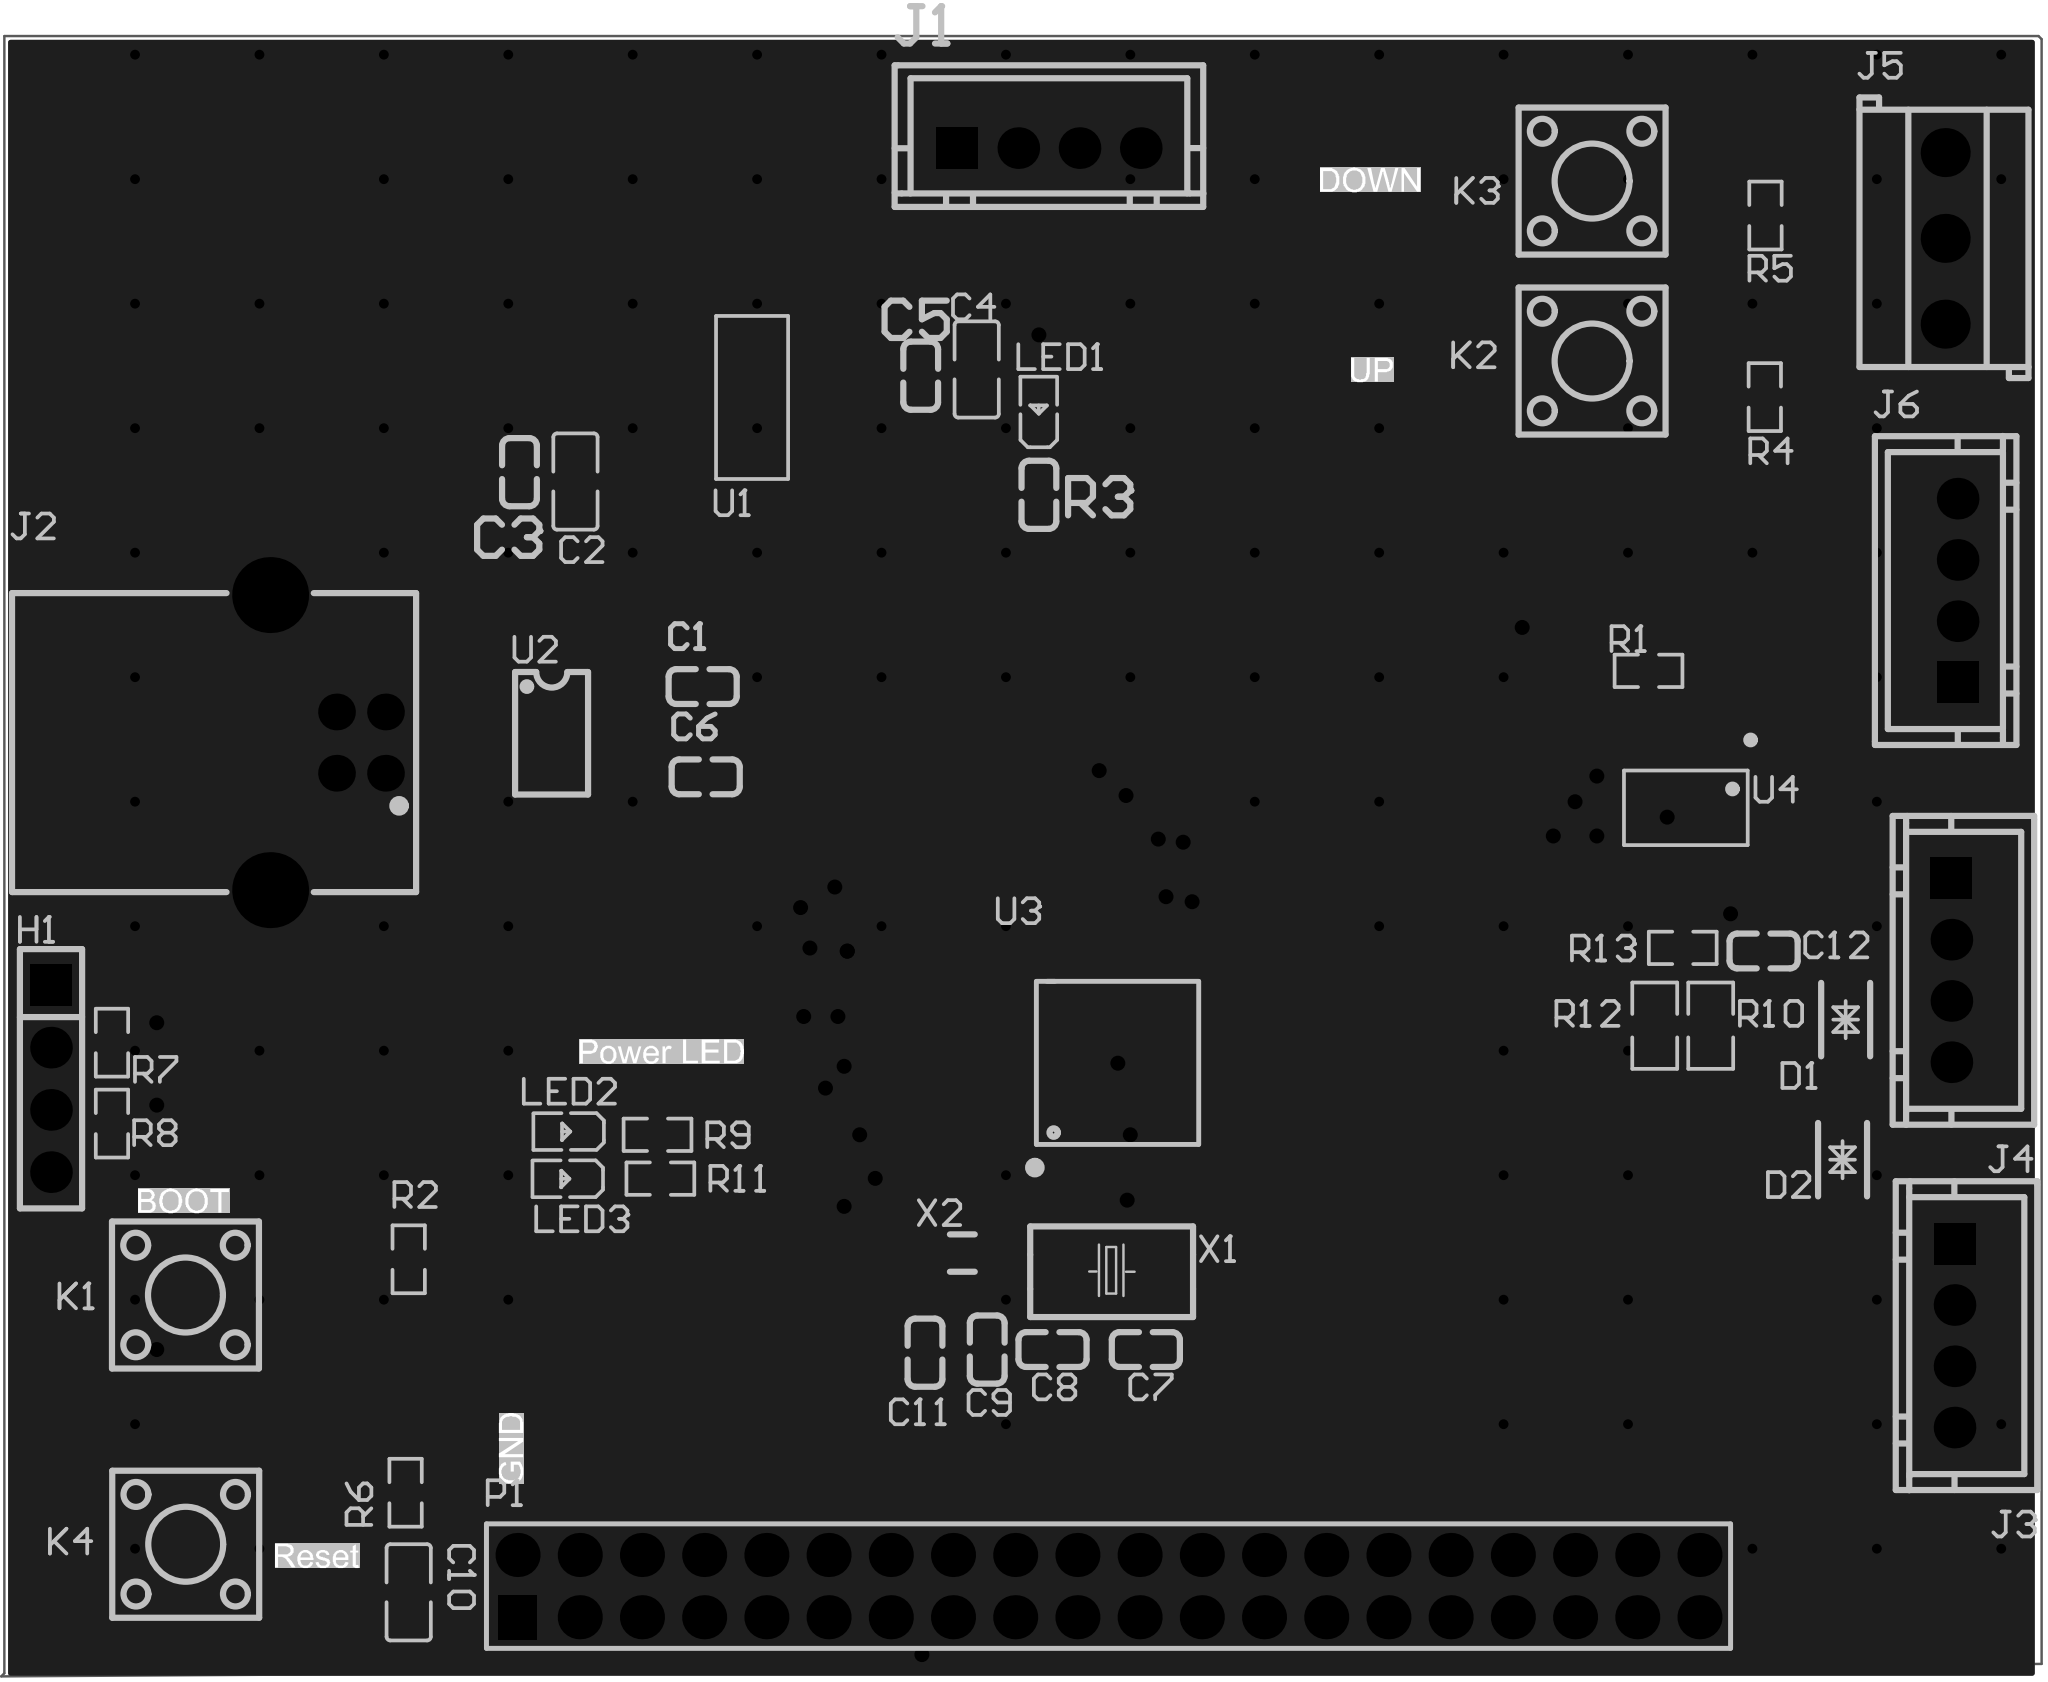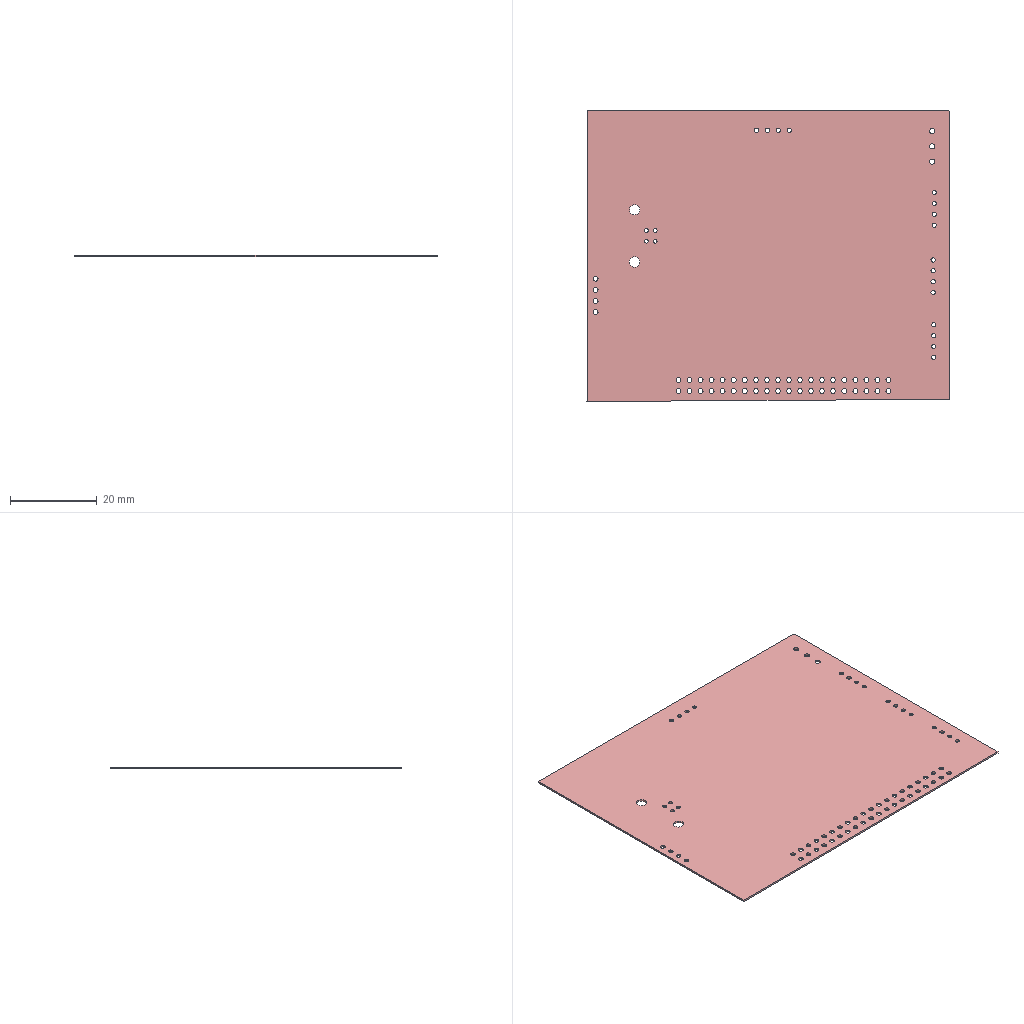Circuit board layout | Altium Designer | box 83.3 x 66.9 x 0.4 mm
Layer stack:
# Altium Designer layer stack of  (unit mm; dielectric type: 0 none, 1 core, 2 prepreg, 3 surface material)
index,name,kind,layer,copper_thickness_mm,dielectric_type,dielectric_thickness_mm,dielectric_material,dielectric_constant
0,Top Paste Mask Layer,other,,,,,,
1,Top Silkscreen Layer,other,,,,,,
2,Top Solder Mask Layer,dielectric,,,3,0.0102,Solder Resist,3.5
3,Top Layer,copper,Top Layer,0.0356,,,,
4,Dielectric 1,dielectric,,,3,0.32,FR-4,4.8
5,Bottom Layer,copper,Bottom Layer,0.0356,,,,
6,Bottom Solder Mask Layer,dielectric,,,3,0.0102,Solder Resist,3.5
7,Bottom Silkscreen Layer,other,,,,,,
8,Bottom Paste Mask Layer,other,,,,,,
# drill layer pairs: low layer,high layer
drill_pair,Top Layer,Bottom Layer
Part placement:
Designator,Comment,Layer,Footprint,Center-X(mm),Center-Y(mm),Rotation
C5,CC0603KRX7R9BB104,TopLayer,C0603_-_duplicate,113.743,129.398,270
C3,CC0603KRX7R9BB104,TopLayer,C0603_-_duplicate,97.36,125.461,270
R3,0603WAF1001T5E,TopLayer,C0603_-_duplicate,118.57,124.538,90
J1,XH-4A,TopLayer,XH-4A,118.979,138.684,0
C6,CC0603KRX7R9BB104,TopLayer,C0603_-_duplicate,104.964,113.03,180
C1,CC0603KRX7R9BB104,TopLayer,C0603_-_duplicate,104.84,116.713,0
X2,X50328MSB2GI,TopLayer,FC-135R_L3.2-W1.5,115.443,93.599,180
X1,Q13FC1350000400,TopLayer,CRYSTAL-SMD_L5.0-W3.2,121.539,92.837,180
U1,AMS1117-3.3,TopLayer,SOT-223-3_L6.5-W3.4-P2.30-LS7.0-BR,106.758,128.509,180
U4,SP3485EEN,TopLayer,485SOP-8_L5.0-W4.0-P1.27-LS6.0-BL,144.985,111.767,180
U3,STM32F103C8T6,TopLayer,LQFP-48_L7.0-W7.0-P0.50-LS9.0-BL,121.793,101.346,0
U2,CH340N_C2977777,TopLayer,SOP-8_L4.9-W3.9-P1.27-LS6.0-BL,98.679,114.808,270
R11,0603WAF1001T5E,TopLayer,R06031k,103.113,96.636,180
R8,0603WAF4701T5E,TopLayer,R06034.7k,80.721,98.882,90
R7,0603WAF4701T5E,TopLayer,R06034.7k,80.721,102.184,90
R9,0603WAF1001T5E,TopLayer,R06031k,102.997,98.425,180
R5,0603WAF1002T5E,TopLayer,电阻R0603,148.237,135.933,270
R2,0603WAF1002T5E,TopLayer,电阻R0603,92.837,93.345,270
R6,0603WAF1002T5E,TopLayer,电阻R0603,92.71,83.82,270
R4,0603WAF1002T5E,TopLayer,电阻R0603,148.209,128.524,270
R1,0603WAF1002T5E,TopLayer,电阻R0603,143.461,117.355,180
R12,0805W8F200JT5E,TopLayer,R0805,143.715,102.877,270
R13,0603WAF1200T5E,TopLayer,R0603_-_duplicate,144.858,106.052,0
R10,0805W8F200JT5E,TopLayer,R0805,146.001,102.877,270
P1,Header-Male-2.54_2x20,TopLayer,HDR-TH_40P-P2.54-V-M-R2-C20-S2.54,121.412,80.01,0
LED3,FC-D1608HGK-572C,TopLayer,LED0603-RD,99.282,96.636,180
LED2,FC-D1608HGK-572C,TopLayer,LED0603-RD,99.318,98.563,180
LED1,FC-D1608HGK-572C,TopLayer,LED0603-RD,118.57,127.967,90
K3,KH-6X6X5H-STM,TopLayer,复位按键,141.157,137.339,180
K4,KH-6X6X5H-STM,TopLayer,复位按键,83.733,81.719,180
K1,KH-6X6X5H-STM,TopLayer,按键,83.722,91.888,0
K2,KH-6X6X5H-STM,TopLayer,复位按键,141.157,129.996,180
J5,KF350-3.5-3P,TopLayer,KF350-3.5-3P,155.575,135.001,90
J6,XH-4A,TopLayer,XH-4A,156.083,120.63,90
J4,XH-4A,TopLayer,XH-4A,155.829,105.136,270
J3,XH-4A,TopLayer,XH-4A,155.956,90.23,270
J2,USB-B-Female-90,TopLayer,USB-B_TH_USB-B-FEMALE-90,89.535,114.427,270
H1,PM254V-11-04-H85,TopLayer,排母4p,78.232,100.711,270
D2,SMF6.0CA_C2990473,TopLayer,瞬态二极管,151.384,97.409,90
D1,SMF6.0CA_C2990473,TopLayer,瞬态二极管,151.511,103.124,90
C11,CL10C200JB8NNNC,TopLayer,C0603c20pf,113.919,89.535,90
C9,CL10C200JB8NNNC,TopLayer,C0603c20pf,116.459,89.662,90
C8,CL10C200JB8NNNC,TopLayer,C0603c20pf,119.126,89.662,0
C10,CL21A106KAYNNNE,TopLayer,C0805,92.837,79.756,90
C7,CL10C200JB8NNNC,TopLayer,C0603c20pf,122.936,89.662,0
C2,CL21A106KAYNNNE,TopLayer,C0805,99.646,125.08,90
C4,CL21A106KAYNNNE,TopLayer,C0805,116.029,129.652,270
C12,CC0603KRX7R9BB104,TopLayer,C0603_-_duplicate,148.16,105.925,0
Pad and via stacks:
# Altium Designer via and pad stacks of  (unit mm). Each distinct definition once, with the count of objects using it.
# via: kind,start_layer,end_layer,hole_mm,diameter_mm,mode(0 simple;1 top-mid-bottom;2 full stack),diameter_per_layer,count,example_net
# pad: kind,layer,hole_mm,hole_type(0 round;1 square;2 slot),plating,top_size,top_shape(1 round;2 rect;3 octagon;9 rounded rect),mid_size,bottom_size,mode,footprint,size_per_layer,count,example
pad,Top Layer,0,0,plated,0.8x0.9,2,0.8x0.9,0.8x0.9,0,C0603 - duplicate,,12,C5.2
pad,Top Layer,0,0,plated,1.8x1,2,1.8x1,1.8x1,0,FC-135R_L3.2-W1.5,,2,X2.2
pad,Top Layer,0,0,plated,1.9x2.4,2,1.9x2.4,1.9x2.4,0,CRYSTAL-SMD_L5.0-W3.2,,2,X1.1
pad,Top Layer,0,0,plated,2.34x3.6,2,2.34x3.6,2.34x3.6,0,SOT-223-3_L6.5-W3.4-P2.30-LS7.0-BR,,1,U1.4
pad,Top Layer,0,0,plated,2.5x1.1,2,2.5x1.1,2.5x1.1,0,SOT-223-3_L6.5-W3.4-P2.30-LS7.0-BR,,3,U1.3
pad,Top Layer,0,0,plated,0.574x2.035,1,0.574x2.035,0.574x2.035,0,485SOP-8_L5.0-W4.0-P1.27-LS6.0-BL,,8,U4.1
pad,Top Layer,0,0,plated,0.27x1.5,1,0.27x1.5,0.27x1.5,0,LQFP-48_L7.0-W7.0-P0.50-LS9.0-BL,,24,U3.1
pad,Top Layer,0,0,plated,1.5x0.27,1,1.5x0.27,1.5x0.27,0,LQFP-48_L7.0-W7.0-P0.50-LS9.0-BL,,24,U3.13
pad,Top Layer,0,0,plated,0.63x1.865,1,0.63x1.865,0.63x1.865,0,SOP-8_L4.9-W3.9-P1.27-LS6.0-BL,,8,U2.1
pad,Top Layer,0,0,plated,0.8065x0.864,2,0.8065x0.864,0.8065x0.864,0,R06031k,,4,R11.1
pad,Top Layer,0,0,plated,0.8065x0.864,2,0.8065x0.864,0.8065x0.864,0,R06034.7k,,4,R8.1
pad,Top Layer,0,0,plated,0.8065x0.864,2,0.8065x0.864,0.8065x0.864,0,\u00B5\u00E7\u00D7\u00E8R0603,,10,R5.2
pad,Top Layer,0,0,plated,1.133x1.377,2,1.133x1.377,1.133x1.377,0,R0805,,4,R12.1
pad,Top Layer,0,0,plated,0.8065x0.864,2,0.8065x0.864,0.8065x0.864,0,R0603 - duplicate,,2,R13.2
pad,Top Layer,0,0,plated,0.8x0.8,2,0.8x0.8,0.8x0.8,0,LED0603-RD,,6,LED3.1
pad,Top Layer,0,0,plated,2.3x1.5,2,2.3x1.5,2.3x1.5,0,\u00B8\u00B4\u00CE\u00BB\u00B0\u00B4\u00BC\u00FC,,12,K3.4
pad,Top Layer,0,0,plated,2.3x1.5,2,2.3x1.5,2.3x1.5,0,\u00B0\u00B4\u00BC\u00FC,,4,K1.4
pad,Top Layer,0,0,plated,1.2x1.4,2,1.2x1.4,1.2x1.4,0,\u00CB\u00B2\u00CC\u00AC\u00B6\u00FE\u00BC\u00AB\u00B9\u00DC,,4,D2.2
pad,Top Layer,0,0,plated,0.8x0.9,2,0.8x0.9,0.8x0.9,0,C0603c20pf,,8,C11.2
pad,Top Layer,0,0,plated,1.41x1.35,2,1.41x1.35,1.41x1.35,0,C0805,,6,C10.2
pad,Multi-Layer,1,0,plated,1.7x1.7,1,1.7x1.7,1.7x1.7,0,XH-4A,,12,J1.4
pad,Multi-Layer,1,0,plated,1.7x1.7,2,1.7x1.7,1.7x1.7,0,XH-4A,,4,J1.1
pad,Multi-Layer,1.1,0,plated,1.8x1.8,1,1.8x1.8,1.8x1.8,0,HDR-TH_40P-P2.54-V-M-R2-C20-S2.54,,39,P1.40
pad,Multi-Layer,1.1,0,plated,1.575x1.8,2,1.575x1.8,1.575x1.8,0,HDR-TH_40P-P2.54-V-M-R2-C20-S2.54,,1,P1.1
pad,Multi-Layer,1.2,0,plated,2x2,1,2x2,2x2,0,KF350-3.5-3P,,3,J5.3
pad,Multi-Layer,2.4,0,plated,3.1x3.1,1,3.1x3.1,3.1x3.1,0,USB-B_TH_USB-B-FEMALE-90,,2,J2.6
pad,Multi-Layer,0.9,0,plated,1.5x1.5,1,1.5x1.5,1.5x1.5,0,USB-B_TH_USB-B-FEMALE-90,,4,J2.2
pad,Multi-Layer,1.1,0,plated,1.7x1.7,1,1.7x1.7,1.7x1.7,0,\u00C5\u00C5\u00C4\u00B84p,,3,H1.4
pad,Multi-Layer,1.1,0,plated,1.7x1.7,2,1.7x1.7,1.7x1.7,0,\u00C5\u00C5\u00C4\u00B84p,,1,H1.1
via,Top Layer,Bottom Layer,0.3048,0.61,0,,33,PB5
via,Top Layer,Bottom Layer,0.2997,0.4,0,,130,GND
Copper pours:
name,layer,net,type(0 solid;1 hatched;2 none)
Top Layer-GND,Top Layer,GND,0
Bottom Layer-GND,Bottom Layer,GND,0
Design rules, without the lines most boards share:
# Altium Designer design rules of  (exported by Altium Designer, unit mm)
# columns: name | kind | enabled | priority | scope1 | scope2 | descriptor | typed fields (field=value)
ComponentClearance_1 | 24 | enabled | 1 | All | All | Component Clearance Constraint ( Horizontal Gap = 10mil, Vertical Gap = 10mil ) (All),(All)  | gap=0.254
Clearance | 0 | enabled | 1 | All | All | Clearance Constraint (Gap=6mil) (All),(All) | gap=0.1524
Clearance_1 | 63 | enabled | 1 | All | All | Board Clearance Constraint (Gap=0mil) (All) |
ComponentClearance | 52 | enabled | 1 | All | All | Hole To Hole Clearance (Gap=0mil) (All),(All) | gap=0
Width | 2 | enabled | 1 | All | All | Width Constraint (Min=6mil) (Max=100mil) (Preferred=10mil) (All) |
DiffPairsRouting | 51 | enabled | 1 | All | All | Differential Pairs Uncoupled Length using the Gap Constraints (Min=10mil) (Max=10mil) (Prefered=10mil)  and Width Constraints (Min=15mil) (Max=15mil) (Prefered=15mil) (All) |
RoutingVias | 11 | enabled | 1 | All | All | Routing Via (MinHoleWidth=11.811mil) (MaxHoleWidth=39.37mil) (PreferredHoleWidth=11.811mil) (MinWidth=15.748mil) (MaxWidth=50mil) (PreferedWidth=15.748mil) (All) | via_min_hole=0.3 via_max_hole=1 via_preferred_diameter=0.4 via_preferred_hole=0.3
PlaneConnect_1 | 6 | disabled | 1 | All | All | Power Plane Connect Rule(Direct Connect )(Expansion=20mil) (Conductor Width=10mil) (Air Gap=10mil) (Entries=4) (Disabled)(All) | relief_conductor_width=0.254 relief_entries=4 relief_expansion=0.508
PlaneConnect | 6 | enabled | 2 | All | All | Power Plane Connect Rule(Relief Connect )(Expansion=20mil) (Conductor Width=10mil) (Air Gap=10mil) (Entries=4) (All) | relief_conductor_width=0.254 relief_entries=4 relief_expansion=0.508
PolygonConnect | 20 | enabled | 1 | (InNet('GND')) | All | Polygon Connect Rule(Relief Connect )(Conductor Width=10mil) (Relief Angle=90 Angle) (Entries=4) (Air Gap Width=10mil) ((InNet('GND'))),(All) | connect_style(0=relief,1=direct,2=none)=0 relief_conductor_width=0.254 relief_entries=4
PasteMaskExpansion | 14 | enabled | 1 | All | All | Paste Mask Expansion (Expansion =0mil) (All) | expansion=0
SolderMaskExpansion | 13 | enabled | 1 | All | All | Solder Mask Expansion (Expansion =4mil) (All) | expansion=0.1016